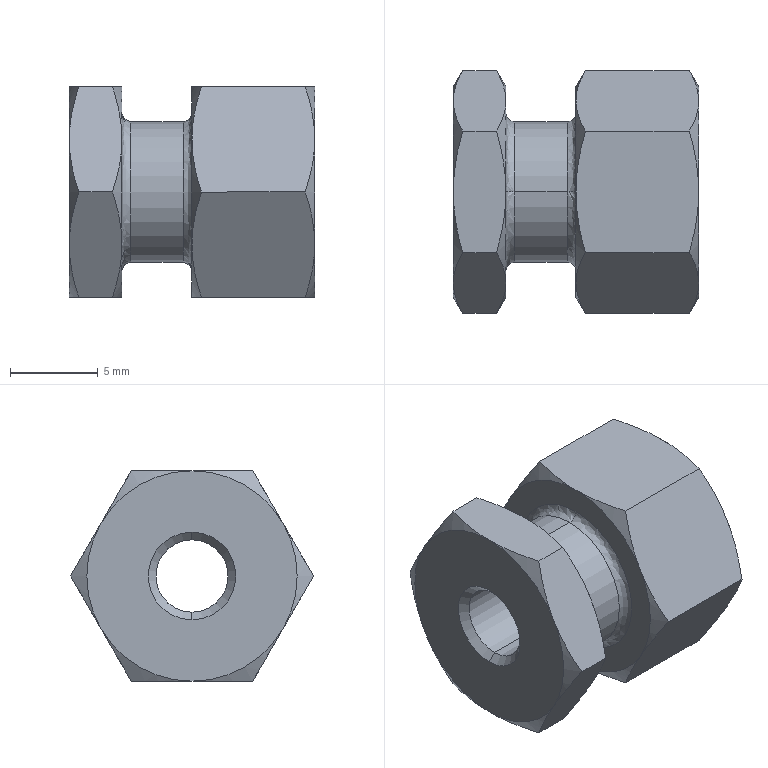Part | STEP file | QA-KFJR5-0.8-4 | 1 solid | 52 faces | box 14 x 13.856 x 12 mm | volume 1253 mm3 | cone 28 | plane 16 | spline 4 | cylinder 4 | commonest cylinder face diameters 4.134 x2 8 x2